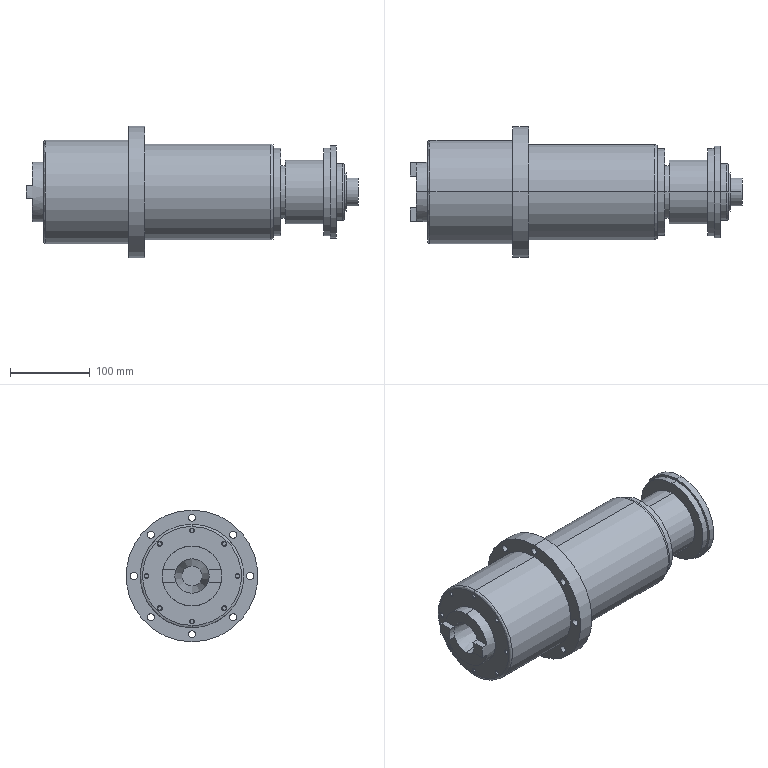Part | SolidWorks | features BaseBody 1 | 1 solid | 115 faces | box 416 x 165 x 165 mm | volume 4108443 mm3 | cylinder 60 | plane 31 | cone 20 | spline 4 | commonest cylinder face diameters 5 x16 9 x16 120 x4 35 x2 43.1 x2 48 x2